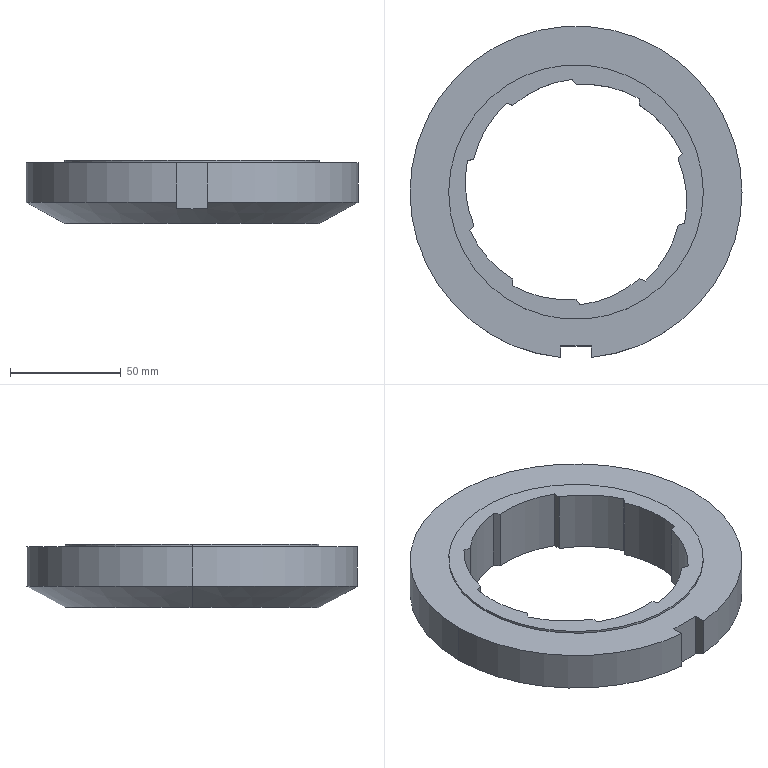Part | SolidWorks | features BaseBody 1, ICE 1 | 1 solid | 36 faces | box 150 x 149.673 x 28.6 mm | volume 237488 mm3 | cylinder 18 | plane 16 | cone 2 | commonest cylinder face diameters 100 x11 115 x4 150 x3
STEP:
#1=CARTESIAN_POINT('',(463.731,234.744,-713.193));
#2=VERTEX_POINT('',#1);
#3=CARTESIAN_POINT('',(578.731,234.744,-713.193));
#4=VERTEX_POINT('',#3);
#5=CARTESIAN_POINT('',(521.231,234.744,-713.193));
#6=DIRECTION('',(0.,0.,-1.));
#7=DIRECTION('',(-1.,0.,0.));
#8=AXIS2_PLACEMENT_3D('',#5,#6,#7);
#9=CIRCLE('',#8,57.5);
#10=EDGE_CURVE('',#2,#4,#9,.T.);
#11=ORIENTED_EDGE('',*,*,#10,.F.);
#12=CARTESIAN_POINT('',(446.231,234.744,-703.693));
#13=VERTEX_POINT('',#12);
#14=CARTESIAN_POINT('',(463.731,234.744,-713.193));
#15=DIRECTION('',(-0.8789,0.,0.4771));
#16=VECTOR('',#15,1000.);
#17=LINE('',#14,#16);
#18=EDGE_CURVE('',#2,#13,#17,.T.);
#19=ORIENTED_EDGE('',*,*,#18,.T.);
#20=CARTESIAN_POINT('',(596.231,234.744,-703.693));
#21=VERTEX_POINT('',#20);
#22=CARTESIAN_POINT('',(521.231,234.744,-703.693));
#23=DIRECTION('',(0.,0.,-1.));
#24=DIRECTION('',(-1.,0.,0.));
#25=AXIS2_PLACEMENT_3D('',#22,#23,#24);
#26=CIRCLE('',#25,75.);
#27=EDGE_CURVE('',#13,#21,#26,.T.);
#28=ORIENTED_EDGE('',*,*,#27,.T.);
#29=CARTESIAN_POINT('',(578.731,234.744,-713.193));
#30=DIRECTION('',(0.8789,0.,0.4771));
#31=VECTOR('',#30,1000.);
#32=LINE('',#29,#31);
#33=EDGE_CURVE('',#4,#21,#32,.T.);
#34=ORIENTED_EDGE('',*,*,#33,.F.);
#35=EDGE_LOOP('',(#11,#19,#28,#34));
#36=FACE_OUTER_BOUND('',#35,.T.);
#37=CARTESIAN_POINT('',(521.231,234.744,-713.193));
#38=DIRECTION('',(0.,0.,1.));
#39=DIRECTION('',(1.,0.,0.));
#40=AXIS2_PLACEMENT_3D('',#37,#38,#39);
#41=CONICAL_SURFACE('',#40,57.5,1.073);
#42=ADVANCED_FACE('',(#36),#41,.T.);
#43=CARTESIAN_POINT('',(578.731,234.744,-685.693));
#44=VERTEX_POINT('',#43);
#45=CARTESIAN_POINT('',(463.731,234.744,-685.693));
#46=VERTEX_POINT('',#45);
#47=CARTESIAN_POINT('',(521.231,234.744,-685.693));
#48=DIRECTION('',(0.,0.,1.));
#49=DIRECTION('',(1.,0.,0.));
#50=AXIS2_PLACEMENT_3D('',#47,#48,#49);
#51=CIRCLE('',#50,57.5);
#52=EDGE_CURVE('',#44,#46,#51,.T.);
#53=ORIENTED_EDGE('',*,*,#52,.T.);
#54=CARTESIAN_POINT('',(463.731,234.744,-684.693));
#55=VERTEX_POINT('',#54);
#56=CARTESIAN_POINT('',(463.731,234.744,-685.693));
#57=DIRECTION('',(0.,0.,1.));
#58=VECTOR('',#57,1000.);
#59=LINE('',#56,#58);
#60=EDGE_CURVE('',#46,#55,#59,.T.);
#61=ORIENTED_EDGE('',*,*,#60,.T.);
#62=CARTESIAN_POINT('',(578.731,234.744,-684.693));
#63=VERTEX_POINT('',#62);
#64=CARTESIAN_POINT('',(521.231,234.744,-684.693));
#65=DIRECTION('',(0.,0.,1.));
#66=DIRECTION('',(1.,0.,0.));
#67=AXIS2_PLACEMENT_3D('',#64,#65,#66);
#68=CIRCLE('',#67,57.5);
#69=EDGE_CURVE('',#63,#55,#68,.T.);
#70=ORIENTED_EDGE('',*,*,#69,.F.);
#71=CARTESIAN_POINT('',(578.731,234.744,-685.693));
#72=DIRECTION('',(0.,0.,1.));
#73=VECTOR('',#72,1000.);
#74=LINE('',#71,#73);
#75=EDGE_CURVE('',#44,#63,#74,.T.);
#76=ORIENTED_EDGE('',*,*,#75,.F.);
#77=EDGE_LOOP('',(#53,#61,#70,#76));
#78=FACE_OUTER_BOUND('',#77,.T.);
#79=CARTESIAN_POINT('',(521.231,234.744,-685.693));
#80=DIRECTION('',(0.,0.,1.));
#81=DIRECTION('',(1.,0.,0.));
#82=AXIS2_PLACEMENT_3D('',#79,#80,#81);
#83=CYLINDRICAL_SURFACE('',#82,57.5);
#84=ADVANCED_FACE('',(#78),#83,.T.);
#85=ORIENTED_EDGE('',*,*,#27,.F.);
#86=CARTESIAN_POINT('',(446.231,234.744,-685.693));
#87=VERTEX_POINT('',#86);
#88=CARTESIAN_POINT('',(446.231,234.744,-714.693));
#89=DIRECTION('',(0.,0.,1.));
#90=VECTOR('',#89,1000.);
#91=LINE('',#88,#90);
#92=EDGE_CURVE('',#13,#87,#91,.T.);
#93=ORIENTED_EDGE('',*,*,#92,.T.);
#94=CARTESIAN_POINT('',(596.231,234.744,-685.693));
#95=VERTEX_POINT('',#94);
#96=CARTESIAN_POINT('',(521.231,234.744,-685.693));
#97=DIRECTION('',(0.,0.,1.));
#98=DIRECTION('',(1.,0.,0.));
#99=AXIS2_PLACEMENT_3D('',#96,#97,#98);
#100=CIRCLE('',#99,75.);
#101=EDGE_CURVE('',#95,#87,#100,.T.);
#102=ORIENTED_EDGE('',*,*,#101,.F.);
#103=CARTESIAN_POINT('',(596.231,234.744,-714.693));
#104=DIRECTION('',(0.,0.,1.));
#105=VECTOR('',#104,1000.);
#106=LINE('',#103,#105);
#107=EDGE_CURVE('',#21,#95,#106,.T.);
#108=ORIENTED_EDGE('',*,*,#107,.F.);
#109=EDGE_LOOP('',(#85,#93,#102,#108));
#110=FACE_OUTER_BOUND('',#109,.T.);
#111=CARTESIAN_POINT('',(521.231,234.744,-714.693));
#112=DIRECTION('',(0.,0.,1.));
#113=DIRECTION('',(1.,0.,0.));
#114=AXIS2_PLACEMENT_3D('',#111,#112,#113);
#115=CYLINDRICAL_SURFACE('',#114,75.);
#116=ADVANCED_FACE('',(#110),#115,.T.);
#117=CARTESIAN_POINT('',(528.231,160.071,-703.693));
#118=VERTEX_POINT('',#117);
#119=CARTESIAN_POINT('',(521.231,234.744,-703.693));
#120=DIRECTION('',(0.,0.,-1.));
#121=DIRECTION('',(-1.,0.,0.));
#122=AXIS2_PLACEMENT_3D('',#119,#120,#121);
#123=CIRCLE('',#122,75.);
#124=EDGE_CURVE('',#21,#118,#123,.T.);
#125=ORIENTED_EDGE('',*,*,#124,.F.);
#126=ORIENTED_EDGE('',*,*,#107,.T.);
#127=CARTESIAN_POINT('',(528.231,160.071,-685.693));
#128=VERTEX_POINT('',#127);
#129=CARTESIAN_POINT('',(521.231,234.744,-685.693));
#130=DIRECTION('',(0.,0.,1.));
#131=DIRECTION('',(1.,0.,0.));
#132=AXIS2_PLACEMENT_3D('',#129,#130,#131);
#133=CIRCLE('',#132,75.);
#134=EDGE_CURVE('',#128,#95,#133,.T.);
#135=ORIENTED_EDGE('',*,*,#134,.F.);
#136=CARTESIAN_POINT('',(528.231,160.071,-714.693));
#137=DIRECTION('',(0.,0.,-1.));
#138=VECTOR('',#137,1000.);
#139=LINE('',#136,#138);
#140=EDGE_CURVE('',#128,#118,#139,.T.);
#141=ORIENTED_EDGE('',*,*,#140,.T.);
#142=EDGE_LOOP('',(#125,#126,#135,#141));
#143=FACE_OUTER_BOUND('',#142,.T.);
#144=CARTESIAN_POINT('',(521.231,234.744,-714.693));
#145=DIRECTION('',(0.,0.,1.));
#146=DIRECTION('',(1.,0.,0.));
#147=AXIS2_PLACEMENT_3D('',#144,#145,#146);
#148=CYLINDRICAL_SURFACE('',#147,75.);
#149=ADVANCED_FACE('',(#143),#148,.T.);
#150=CARTESIAN_POINT('',(471.242,239.027,-684.693));
#151=VERTEX_POINT('',#150);
#152=CARTESIAN_POINT('',(472.206,248.801,-684.693));
#153=VERTEX_POINT('',#152);
#154=CARTESIAN_POINT('',(521.242,239.027,-684.693));
#155=DIRECTION('',(0.,0.,-1.));
#156=DIRECTION('',(-1.,0.,0.));
#157=AXIS2_PLACEMENT_3D('',#154,#155,#156);
#158=CIRCLE('',#157,50.);
#159=EDGE_CURVE('',#151,#153,#158,.T.);
#160=ORIENTED_EDGE('',*,*,#159,.F.);
#161=CARTESIAN_POINT('',(471.242,239.027,-713.293));
#162=VERTEX_POINT('',#161);
#163=CARTESIAN_POINT('',(471.242,239.027,-608.693));
#164=DIRECTION('',(0.,0.,-1.));
#165=VECTOR('',#164,1000.);
#166=LINE('',#163,#165);
#167=EDGE_CURVE('',#151,#162,#166,.T.);
#168=ORIENTED_EDGE('',*,*,#167,.T.);
#169=CARTESIAN_POINT('',(472.206,248.801,-713.293));
#170=VERTEX_POINT('',#169);
#171=CARTESIAN_POINT('',(521.242,239.027,-713.293));
#172=DIRECTION('',(0.,0.,1.));
#173=DIRECTION('',(-1.,0.,0.));
#174=AXIS2_PLACEMENT_3D('',#171,#172,#173);
#175=CIRCLE('',#174,50.);
#176=EDGE_CURVE('',#170,#162,#175,.T.);
#177=ORIENTED_EDGE('',*,*,#176,.F.);
#178=CARTESIAN_POINT('',(472.206,248.801,-608.693));
#179=DIRECTION('',(0.,0.,-1.));
#180=VECTOR('',#179,1000.);
#181=LINE('',#178,#180);
#182=EDGE_CURVE('',#153,#170,#181,.T.);
#183=ORIENTED_EDGE('',*,*,#182,.F.);
#184=EDGE_LOOP('',(#160,#168,#177,#183));
#185=FACE_OUTER_BOUND('',#184,.T.);
#186=CARTESIAN_POINT('',(521.242,239.027,-608.693));
#187=DIRECTION('',(0.,0.,-1.));
#188=DIRECTION('',(-1.,0.,0.));
#189=AXIS2_PLACEMENT_3D('',#186,#187,#188);
#190=CYLINDRICAL_SURFACE('',#189,50.);
#191=ADVANCED_FACE('',(#185),#190,.F.);
#192=ORIENTED_EDGE('',*,*,#10,.T.);
#193=CARTESIAN_POINT('',(578.731,234.744,-713.293));
#194=VERTEX_POINT('',#193);
#195=CARTESIAN_POINT('',(578.731,234.744,-713.193));
#196=DIRECTION('',(0.,0.,-1.));
#197=VECTOR('',#196,1000.);
#198=LINE('',#195,#197);
#199=EDGE_CURVE('',#4,#194,#198,.T.);
#200=ORIENTED_EDGE('',*,*,#199,.T.);
#201=CARTESIAN_POINT('',(463.731,234.744,-713.293));
#202=VERTEX_POINT('',#201);
#203=CARTESIAN_POINT('',(521.231,234.744,-713.293));
#204=DIRECTION('',(0.,0.,-1.));
#205=DIRECTION('',(-1.,0.,0.));
#206=AXIS2_PLACEMENT_3D('',#203,#204,#205);
#207=CIRCLE('',#206,57.5);
#208=EDGE_CURVE('',#202,#194,#207,.T.);
#209=ORIENTED_EDGE('',*,*,#208,.F.);
#210=CARTESIAN_POINT('',(463.731,234.744,-713.193));
#211=DIRECTION('',(0.,0.,-1.));
#212=VECTOR('',#211,1000.);
#213=LINE('',#210,#212);
#214=EDGE_CURVE('',#2,#202,#213,.T.);
#215=ORIENTED_EDGE('',*,*,#214,.F.);
#216=EDGE_LOOP('',(#192,#200,#209,#215));
#217=FACE_OUTER_BOUND('',#216,.T.);
#218=CARTESIAN_POINT('',(521.231,234.744,-713.193));
#219=DIRECTION('',(0.,0.,-1.));
#220=DIRECTION('',(-1.,0.,0.));
#221=AXIS2_PLACEMENT_3D('',#218,#219,#220);
#222=CYLINDRICAL_SURFACE('',#221,57.5);
#223=ADVANCED_FACE('',(#217),#222,.T.);
#224=ORIENTED_EDGE('',*,*,#199,.F.);
#225=CARTESIAN_POINT('',(521.231,234.744,-713.193));
#226=DIRECTION('',(0.,0.,-1.));
#227=DIRECTION('',(-1.,0.,0.));
#228=AXIS2_PLACEMENT_3D('',#225,#226,#227);
#229=CIRCLE('',#228,57.5);
#230=EDGE_CURVE('',#4,#2,#229,.T.);
#231=ORIENTED_EDGE('',*,*,#230,.T.);
#232=ORIENTED_EDGE('',*,*,#214,.T.);
#233=CARTESIAN_POINT('',(521.231,234.744,-713.293));
#234=DIRECTION('',(0.,0.,-1.));
#235=DIRECTION('',(-1.,0.,0.));
#236=AXIS2_PLACEMENT_3D('',#233,#234,#235);
#237=CIRCLE('',#236,57.5);
#238=EDGE_CURVE('',#194,#202,#237,.T.);
#239=ORIENTED_EDGE('',*,*,#238,.F.);
#240=EDGE_LOOP('',(#224,#231,#232,#239));
#241=FACE_OUTER_BOUND('',#240,.T.);
#242=CARTESIAN_POINT('',(521.231,234.744,-713.193));
#243=DIRECTION('',(0.,0.,-1.));
#244=DIRECTION('',(-1.,0.,0.));
#245=AXIS2_PLACEMENT_3D('',#242,#243,#244);
#246=CYLINDRICAL_SURFACE('',#245,57.5);
#247=ADVANCED_FACE('',(#241),#246,.T.);
#248=CARTESIAN_POINT('',(521.231,186.244,-713.293));
#249=VERTEX_POINT('',#248);
#250=CARTESIAN_POINT('',(523.011,183.775,-713.293));
#251=VERTEX_POINT('',#250);
#252=CARTESIAN_POINT('',(523.011,183.775,-713.293));
#253=DIRECTION('',(0.5848,-0.8112,0.));
#254=VECTOR('',#253,1000.);
#255=LINE('',#252,#254);
#256=EDGE_CURVE('',#249,#251,#255,.T.);
#257=ORIENTED_EDGE('',*,*,#256,.F.);
#258=CARTESIAN_POINT('',(521.231,186.244,-684.693));
#259=VERTEX_POINT('',#258);
#260=CARTESIAN_POINT('',(521.231,186.244,-608.693));
#261=DIRECTION('',(0.,0.,-1.));
#262=VECTOR('',#261,1000.);
#263=LINE('',#260,#262);
#264=EDGE_CURVE('',#259,#249,#263,.T.);
#265=ORIENTED_EDGE('',*,*,#264,.F.);
#266=CARTESIAN_POINT('',(523.011,183.775,-684.693));
#267=VERTEX_POINT('',#266);
#268=CARTESIAN_POINT('',(498.224,218.158,-684.693));
#269=DIRECTION('',(-0.5848,0.8112,0.));
#270=VECTOR('',#269,1000.);
#271=LINE('',#268,#270);
#272=EDGE_CURVE('',#267,#259,#271,.T.);
#273=ORIENTED_EDGE('',*,*,#272,.F.);
#274=CARTESIAN_POINT('',(523.011,183.775,-608.693));
#275=DIRECTION('',(0.,0.,-1.));
#276=VECTOR('',#275,1000.);
#277=LINE('',#274,#276);
#278=EDGE_CURVE('',#267,#251,#277,.T.);
#279=ORIENTED_EDGE('',*,*,#278,.T.);
#280=EDGE_LOOP('',(#257,#265,#273,#279));
#281=FACE_OUTER_BOUND('',#280,.T.);
#282=CARTESIAN_POINT('',(523.011,183.775,-608.693));
#283=DIRECTION('',(-0.8112,-0.5848,0.));
#284=DIRECTION('',(-0.5848,0.8112,0.));
#285=AXIS2_PLACEMENT_3D('',#282,#283,#284);
#286=PLANE('',#285);
#287=ADVANCED_FACE('',(#281),#286,.F.);
#288=CARTESIAN_POINT('',(492.712,192.463,-713.293));
#289=VERTEX_POINT('',#288);
#290=CARTESIAN_POINT('',(517.16,236.078,-713.293));
#291=DIRECTION('',(0.,0.,1.));
#292=DIRECTION('',(-1.,0.,0.));
#293=AXIS2_PLACEMENT_3D('',#290,#291,#292);
#294=CIRCLE('',#293,50.);
#295=EDGE_CURVE('',#289,#249,#294,.T.);
#296=ORIENTED_EDGE('',*,*,#295,.F.);
#297=CARTESIAN_POINT('',(492.712,192.463,-684.693));
#298=VERTEX_POINT('',#297);
#299=CARTESIAN_POINT('',(492.712,192.463,-608.693));
#300=DIRECTION('',(0.,0.,-1.));
#301=VECTOR('',#300,1000.);
#302=LINE('',#299,#301);
#303=EDGE_CURVE('',#298,#289,#302,.T.);
#304=ORIENTED_EDGE('',*,*,#303,.F.);
#305=CARTESIAN_POINT('',(517.16,236.078,-684.693));
#306=DIRECTION('',(0.,0.,-1.));
#307=DIRECTION('',(-1.,0.,0.));
#308=AXIS2_PLACEMENT_3D('',#305,#306,#307);
#309=CIRCLE('',#308,50.);
#310=EDGE_CURVE('',#259,#298,#309,.T.);
#311=ORIENTED_EDGE('',*,*,#310,.F.);
#312=ORIENTED_EDGE('',*,*,#264,.T.);
#313=EDGE_LOOP('',(#296,#304,#311,#312));
#314=FACE_OUTER_BOUND('',#313,.T.);
#315=CARTESIAN_POINT('',(517.16,236.078,-608.693));
#316=DIRECTION('',(0.,0.,-1.));
#317=DIRECTION('',(-1.,0.,0.));
#318=AXIS2_PLACEMENT_3D('',#315,#316,#317);
#319=CYLINDRICAL_SURFACE('',#318,50.);
#320=ADVANCED_FACE('',(#314),#319,.F.);
#321=CARTESIAN_POINT('',(475.104,219.757,-713.293));
#322=VERTEX_POINT('',#321);
#323=CARTESIAN_POINT('',(473.306,217.301,-713.293));
#324=VERTEX_POINT('',#323);
#325=CARTESIAN_POINT('',(473.306,217.301,-713.293));
#326=DIRECTION('',(-0.5908,-0.8068,0.));
#327=VECTOR('',#326,1000.);
#328=LINE('',#325,#327);
#329=EDGE_CURVE('',#322,#324,#328,.T.);
#330=ORIENTED_EDGE('',*,*,#329,.F.);
#331=CARTESIAN_POINT('',(475.104,219.757,-684.693));
#332=VERTEX_POINT('',#331);
#333=CARTESIAN_POINT('',(475.104,219.757,-608.693));
#334=DIRECTION('',(0.,0.,-1.));
#335=VECTOR('',#334,1000.);
#336=LINE('',#333,#335);
#337=EDGE_CURVE('',#332,#322,#336,.T.);
#338=ORIENTED_EDGE('',*,*,#337,.F.);
#339=CARTESIAN_POINT('',(473.306,217.301,-684.693));
#340=VERTEX_POINT('',#339);
#341=CARTESIAN_POINT('',(498.347,251.5,-684.693));
#342=DIRECTION('',(0.5908,0.8068,0.));
#343=VECTOR('',#342,1000.);
#344=LINE('',#341,#343);
#345=EDGE_CURVE('',#340,#332,#344,.T.);
#346=ORIENTED_EDGE('',*,*,#345,.F.);
#347=CARTESIAN_POINT('',(473.306,217.301,-608.693));
#348=DIRECTION('',(0.,0.,-1.));
#349=VECTOR('',#348,1000.);
#350=LINE('',#347,#349);
#351=EDGE_CURVE('',#340,#324,#350,.T.);
#352=ORIENTED_EDGE('',*,*,#351,.T.);
#353=EDGE_LOOP('',(#330,#338,#346,#352));
#354=FACE_OUTER_BOUND('',#353,.T.);
#355=CARTESIAN_POINT('',(473.306,217.301,-608.693));
#356=DIRECTION('',(-0.8068,0.5908,0.));
#357=DIRECTION('',(0.5908,0.8068,0.));
#358=AXIS2_PLACEMENT_3D('',#355,#356,#357);
#359=PLANE('',#358);
#360=ADVANCED_FACE('',(#354),#359,.F.);
#361=CARTESIAN_POINT('',(492.723,273.981,-713.293));
#362=VERTEX_POINT('',#361);
#363=CARTESIAN_POINT('',(489.832,274.933,-713.293));
#364=VERTEX_POINT('',#363);
#365=CARTESIAN_POINT('',(489.832,274.933,-713.293));
#366=DIRECTION('',(-0.9499,0.3125,0.));
#367=VECTOR('',#366,1000.);
#368=LINE('',#365,#367);
#369=EDGE_CURVE('',#362,#364,#368,.T.);
#370=ORIENTED_EDGE('',*,*,#369,.F.);
#371=CARTESIAN_POINT('',(492.723,273.981,-684.693));
#372=VERTEX_POINT('',#371);
#373=CARTESIAN_POINT('',(492.723,273.981,-608.693));
#374=DIRECTION('',(0.,0.,-1.));
#375=VECTOR('',#374,1000.);
#376=LINE('',#373,#375);
#377=EDGE_CURVE('',#372,#362,#376,.T.);
#378=ORIENTED_EDGE('',*,*,#377,.F.);
#379=CARTESIAN_POINT('',(489.832,274.933,-684.693));
#380=VERTEX_POINT('',#379);
#381=CARTESIAN_POINT('',(530.095,261.686,-684.693));
#382=DIRECTION('',(0.9499,-0.3125,0.));
#383=VECTOR('',#382,1000.);
#384=LINE('',#381,#383);
#385=EDGE_CURVE('',#380,#372,#384,.T.);
#386=ORIENTED_EDGE('',*,*,#385,.F.);
#387=CARTESIAN_POINT('',(489.832,274.933,-608.693));
#388=DIRECTION('',(0.,0.,-1.));
#389=VECTOR('',#388,1000.);
#390=LINE('',#387,#389);
#391=EDGE_CURVE('',#380,#364,#390,.T.);
#392=ORIENTED_EDGE('',*,*,#391,.T.);
#393=EDGE_LOOP('',(#370,#378,#386,#392));
#394=FACE_OUTER_BOUND('',#393,.T.);
#395=CARTESIAN_POINT('',(489.832,274.933,-608.693));
#396=DIRECTION('',(0.3125,0.9499,0.));
#397=DIRECTION('',(0.9499,-0.3125,0.));
#398=AXIS2_PLACEMENT_3D('',#395,#396,#397);
#399=PLANE('',#398);
#400=ADVANCED_FACE('',(#394),#399,.F.);
#401=CARTESIAN_POINT('',(549.738,273.981,-713.293));
#402=VERTEX_POINT('',#401);
#403=CARTESIAN_POINT('',(549.749,277.025,-713.293));
#404=VERTEX_POINT('',#403);
#405=CARTESIAN_POINT('',(549.749,277.025,-713.293));
#406=DIRECTION('',(0.003697,1.,0.));
#407=VECTOR('',#406,1000.);
#408=LINE('',#405,#407);
#409=EDGE_CURVE('',#402,#404,#408,.T.);
#410=ORIENTED_EDGE('',*,*,#409,.F.);
#411=CARTESIAN_POINT('',(549.738,273.981,-684.693));
#412=VERTEX_POINT('',#411);
#413=CARTESIAN_POINT('',(549.738,273.981,-608.693));
#414=DIRECTION('',(0.,0.,-1.));
#415=VECTOR('',#414,1000.);
#416=LINE('',#413,#415);
#417=EDGE_CURVE('',#412,#402,#416,.T.);
#418=ORIENTED_EDGE('',*,*,#417,.F.);
#419=CARTESIAN_POINT('',(549.749,277.025,-684.693));
#420=VERTEX_POINT('',#419);
#421=CARTESIAN_POINT('',(549.593,234.639,-684.693));
#422=DIRECTION('',(-0.003697,-1.,0.));
#423=VECTOR('',#422,1000.);
#424=LINE('',#421,#423);
#425=EDGE_CURVE('',#420,#412,#424,.T.);
#426=ORIENTED_EDGE('',*,*,#425,.F.);
#427=CARTESIAN_POINT('',(549.749,277.025,-608.693));
#428=DIRECTION('',(0.,0.,-1.));
#429=VECTOR('',#428,1000.);
#430=LINE('',#427,#429);
#431=EDGE_CURVE('',#420,#404,#430,.T.);
#432=ORIENTED_EDGE('',*,*,#431,.T.);
#433=EDGE_LOOP('',(#410,#418,#426,#432));
#434=FACE_OUTER_BOUND('',#433,.T.);
#435=CARTESIAN_POINT('',(549.749,277.025,-608.693));
#436=DIRECTION('',(1.,-0.003697,0.));
#437=DIRECTION('',(-0.003697,-1.,0.));
#438=AXIS2_PLACEMENT_3D('',#435,#436,#437);
#439=PLANE('',#438);
#440=ADVANCED_FACE('',(#434),#439,.F.);
#441=CARTESIAN_POINT('',(567.357,219.757,-713.293));
#442=VERTEX_POINT('',#441);
#443=CARTESIAN_POINT('',(570.255,220.686,-713.293));
#444=VERTEX_POINT('',#443);
#445=CARTESIAN_POINT('',(570.255,220.686,-713.293));
#446=DIRECTION('',(0.9522,0.3055,0.));
#447=VECTOR('',#446,1000.);
#448=LINE('',#445,#447);
#449=EDGE_CURVE('',#442,#444,#448,.T.);
#450=ORIENTED_EDGE('',*,*,#449,.F.);
#451=CARTESIAN_POINT('',(567.357,219.757,-684.693));
#452=VERTEX_POINT('',#451);
#453=CARTESIAN_POINT('',(567.357,219.757,-608.693));
#454=DIRECTION('',(0.,0.,-1.));
#455=VECTOR('',#454,1000.);
#456=LINE('',#453,#455);
#457=EDGE_CURVE('',#452,#442,#456,.T.);
#458=ORIENTED_EDGE('',*,*,#457,.F.);
#459=CARTESIAN_POINT('',(570.255,220.686,-684.693));
#460=VERTEX_POINT('',#459);
#461=CARTESIAN_POINT('',(529.895,207.738,-684.693));
#462=DIRECTION('',(-0.9522,-0.3055,0.));
#463=VECTOR('',#462,1000.);
#464=LINE('',#461,#463);
#465=EDGE_CURVE('',#460,#452,#464,.T.);
#466=ORIENTED_EDGE('',*,*,#465,.F.);
#467=CARTESIAN_POINT('',(570.255,220.686,-608.693));
#468=DIRECTION('',(0.,0.,-1.));
#469=VECTOR('',#468,1000.);
#470=LINE('',#467,#469);
#471=EDGE_CURVE('',#460,#444,#470,.T.);
#472=ORIENTED_EDGE('',*,*,#471,.T.);
#473=EDGE_LOOP('',(#450,#458,#466,#472));
#474=FACE_OUTER_BOUND('',#473,.T.);
#475=CARTESIAN_POINT('',(570.255,220.686,-608.693));
#476=DIRECTION('',(0.3055,-0.9522,0.));
#477=DIRECTION('',(-0.9522,-0.3055,0.));
#478=AXIS2_PLACEMENT_3D('',#475,#476,#477);
#479=PLANE('',#478);
#480=ADVANCED_FACE('',(#474),#479,.F.);
#481=CARTESIAN_POINT('',(492.723,195.507,-713.293));
#482=VERTEX_POINT('',#481);
#483=CARTESIAN_POINT('',(518.722,238.216,-713.293));
#484=DIRECTION('',(0.,0.,1.));
#485=DIRECTION('',(-1.,0.,0.));
#486=AXIS2_PLACEMENT_3D('',#483,#484,#485);
#487=CIRCLE('',#486,50.);
#488=EDGE_CURVE('',#324,#482,#487,.T.);
#489=ORIENTED_EDGE('',*,*,#488,.F.);
#490=ORIENTED_EDGE('',*,*,#351,.F.);
#491=CARTESIAN_POINT('',(492.723,195.507,-684.693));
#492=VERTEX_POINT('',#491);
#493=CARTESIAN_POINT('',(518.722,238.216,-684.693));
#494=DIRECTION('',(0.,0.,-1.));
#495=DIRECTION('',(-1.,0.,0.));
#496=AXIS2_PLACEMENT_3D('',#493,#494,#495);
#497=CIRCLE('',#496,50.);
#498=EDGE_CURVE('',#492,#340,#497,.T.);
#499=ORIENTED_EDGE('',*,*,#498,.F.);
#500=CARTESIAN_POINT('',(492.723,195.507,-608.693));
#501=DIRECTION('',(0.,0.,-1.));
#502=VECTOR('',#501,1000.);
#503=LINE('',#500,#502);
#504=EDGE_CURVE('',#492,#482,#503,.T.);
#505=ORIENTED_EDGE('',*,*,#504,.T.);
#506=EDGE_LOOP('',(#489,#490,#499,#505));
#507=FACE_OUTER_BOUND('',#506,.T.);
#508=CARTESIAN_POINT('',(518.722,238.216,-608.693));
#509=DIRECTION('',(0.,0.,-1.));
#510=DIRECTION('',(-1.,0.,0.));
#511=AXIS2_PLACEMENT_3D('',#508,#509,#510);
#512=CYLINDRICAL_SURFACE('',#511,50.);
#513=ADVANCED_FACE('',(#507),#512,.F.);
#514=CARTESIAN_POINT('',(475.104,249.731,-713.293));
#515=VERTEX_POINT('',#514);
#516=CARTESIAN_POINT('',(523.757,238.203,-713.293));
#517=DIRECTION('',(0.,0.,1.));
#518=DIRECTION('',(-1.,0.,0.));
#519=AXIS2_PLACEMENT_3D('',#516,#517,#518);
#520=CIRCLE('',#519,50.);
#521=EDGE_CURVE('',#364,#515,#520,.T.);
#522=ORIENTED_EDGE('',*,*,#521,.F.);
#523=ORIENTED_EDGE('',*,*,#391,.F.);
#524=CARTESIAN_POINT('',(475.104,249.731,-684.693));
#525=VERTEX_POINT('',#524);
#526=CARTESIAN_POINT('',(523.757,238.203,-684.693));
#527=DIRECTION('',(0.,0.,-1.));
#528=DIRECTION('',(-1.,0.,0.));
#529=AXIS2_PLACEMENT_3D('',#526,#527,#528);
#530=CIRCLE('',#529,50.);
#531=EDGE_CURVE('',#525,#380,#530,.T.);
#532=ORIENTED_EDGE('',*,*,#531,.F.);
#533=CARTESIAN_POINT('',(475.104,249.731,-608.693));
#534=DIRECTION('',(0.,0.,-1.));
#535=VECTOR('',#534,1000.);
#536=LINE('',#533,#535);
#537=EDGE_CURVE('',#525,#515,#536,.T.);
#538=ORIENTED_EDGE('',*,*,#537,.T.);
#539=EDGE_LOOP('',(#522,#523,#532,#538));
#540=FACE_OUTER_BOUND('',#539,.T.);
#541=CARTESIAN_POINT('',(523.757,238.203,-608.693));
#542=DIRECTION('',(0.,0.,-1.));
#543=DIRECTION('',(-1.,0.,0.));
#544=AXIS2_PLACEMENT_3D('',#541,#542,#543);
#545=CYLINDRICAL_SURFACE('',#544,50.);
#546=ADVANCED_FACE('',(#540),#545,.F.);
#547=CARTESIAN_POINT('',(521.231,283.244,-713.293));
#548=VERTEX_POINT('',#547);
#549=CARTESIAN_POINT('',(525.301,233.41,-713.293));
#550=DIRECTION('',(0.,0.,1.));
#551=DIRECTION('',(-1.,0.,0.));
#552=AXIS2_PLACEMENT_3D('',#549,#550,#551);
#553=CIRCLE('',#552,50.);
#554=EDGE_CURVE('',#404,#548,#553,.T.);
#555=ORIENTED_EDGE('',*,*,#554,.F.);
#556=ORIENTED_EDGE('',*,*,#431,.F.);
#557=CARTESIAN_POINT('',(521.231,283.244,-684.693));
#558=VERTEX_POINT('',#557);
#559=CARTESIAN_POINT('',(525.301,233.41,-684.693));
#560=DIRECTION('',(0.,0.,-1.));
#561=DIRECTION('',(-1.,0.,0.));
#562=AXIS2_PLACEMENT_3D('',#559,#560,#561);
#563=CIRCLE('',#562,50.);
#564=EDGE_CURVE('',#558,#420,#563,.T.);
#565=ORIENTED_EDGE('',*,*,#564,.F.);
#566=CARTESIAN_POINT('',(521.231,283.244,-608.693));
#567=DIRECTION('',(0.,0.,-1.));
#568=VECTOR('',#567,1000.);
#569=LINE('',#566,#568);
#570=EDGE_CURVE('',#558,#548,#569,.T.);
#571=ORIENTED_EDGE('',*,*,#570,.T.);
#572=EDGE_LOOP('',(#555,#556,#565,#571));
#573=FACE_OUTER_BOUND('',#572,.T.);
#574=CARTESIAN_POINT('',(525.301,233.41,-608.693));
#575=DIRECTION('',(0.,0.,-1.));
#576=DIRECTION('',(-1.,0.,0.));
#577=AXIS2_PLACEMENT_3D('',#574,#575,#576);
#578=CYLINDRICAL_SURFACE('',#577,50.);
#579=ADVANCED_FACE('',(#573),#578,.F.);
#580=CARTESIAN_POINT('',(567.357,249.731,-713.293));
#581=VERTEX_POINT('',#580);
#582=CARTESIAN_POINT('',(521.22,230.461,-713.293));
#583=DIRECTION('',(0.,0.,1.));
#584=DIRECTION('',(-1.,0.,0.));
#585=AXIS2_PLACEMENT_3D('',#582,#583,#584);
#586=CIRCLE('',#585,50.);
#587=EDGE_CURVE('',#444,#581,#586,.T.);
#588=ORIENTED_EDGE('',*,*,#587,.F.);
#589=ORIENTED_EDGE('',*,*,#471,.F.);
#590=CARTESIAN_POINT('',(567.357,249.731,-684.693));
#591=VERTEX_POINT('',#590);
#592=CARTESIAN_POINT('',(521.22,230.461,-684.693));
#593=DIRECTION('',(0.,0.,-1.));
#594=DIRECTION('',(-1.,0.,0.));
#595=AXIS2_PLACEMENT_3D('',#592,#593,#594);
#596=CIRCLE('',#595,50.);
#597=EDGE_CURVE('',#591,#460,#596,.T.);
#598=ORIENTED_EDGE('',*,*,#597,.F.);
#599=CARTESIAN_POINT('',(567.357,249.731,-608.693));
#600=DIRECTION('',(0.,0.,-1.));
#601=VECTOR('',#600,1000.);
#602=LINE('',#599,#601);
#603=EDGE_CURVE('',#591,#581,#602,.T.);
#604=ORIENTED_EDGE('',*,*,#603,.T.);
#605=EDGE_LOOP('',(#588,#589,#598,#604));
#606=FACE_OUTER_BOUND('',#605,.T.);
#607=CARTESIAN_POINT('',(521.22,230.461,-608.693));
#608=DIRECTION('',(0.,0.,-1.));
#609=DIRECTION('',(-1.,0.,0.));
#610=AXIS2_PLACEMENT_3D('',#607,#608,#609);
#611=CYLINDRICAL_SURFACE('',#610,50.);
#612=ADVANCED_FACE('',(#606),#611,.F.);
#613=CARTESIAN_POINT('',(472.206,248.801,-713.293));
#614=DIRECTION('',(-0.9522,-0.3055,0.));
#615=VECTOR('',#614,1000.);
#616=LINE('',#613,#615);
#617=EDGE_CURVE('',#515,#170,#616,.T.);
#618=ORIENTED_EDGE('',*,*,#617,.F.);
#619=ORIENTED_EDGE('',*,*,#537,.F.);
#620=CARTESIAN_POINT('',(512.566,261.75,-684.693));
#621=DIRECTION('',(0.9522,0.3055,0.));
#622=VECTOR('',#621,1000.);
#623=LINE('',#620,#622);
#624=EDGE_CURVE('',#153,#525,#623,.T.);
#625=ORIENTED_EDGE('',*,*,#624,.F.);
#626=ORIENTED_EDGE('',*,*,#182,.T.);
#627=EDGE_LOOP('',(#618,#619,#625,#626));
#628=FACE_OUTER_BOUND('',#627,.T.);
#629=CARTESIAN_POINT('',(472.206,248.801,-608.693));
#630=DIRECTION('',(-0.3055,0.9522,0.));
#631=DIRECTION('',(0.9522,0.3055,0.));
#632=AXIS2_PLACEMENT_3D('',#629,#630,#631);
#633=PLANE('',#632);
#634=ADVANCED_FACE('',(#628),#633,.F.);
#635=CARTESIAN_POINT('',(519.451,285.713,-713.293));
#636=VERTEX_POINT('',#635);
#637=CARTESIAN_POINT('',(519.451,285.713,-713.293));
#638=DIRECTION('',(-0.5848,0.8112,0.));
#639=VECTOR('',#638,1000.);
#640=LINE('',#637,#639);
#641=EDGE_CURVE('',#548,#636,#640,.T.);
#642=ORIENTED_EDGE('',*,*,#641,.F.);
#643=ORIENTED_EDGE('',*,*,#570,.F.);
#644=CARTESIAN_POINT('',(519.451,285.713,-684.693));
#645=VERTEX_POINT('',#644);
#646=CARTESIAN_POINT('',(544.238,251.33,-684.693));
#647=DIRECTION('',(0.5848,-0.8112,0.));
#648=VECTOR('',#647,1000.);
#649=LINE('',#646,#648);
#650=EDGE_CURVE('',#645,#558,#649,.T.);
#651=ORIENTED_EDGE('',*,*,#650,.F.);
#652=CARTESIAN_POINT('',(519.451,285.713,-608.693));
#653=DIRECTION('',(0.,0.,-1.));
#654=VECTOR('',#653,1000.);
#655=LINE('',#652,#654);
#656=EDGE_CURVE('',#645,#636,#655,.T.);
#657=ORIENTED_EDGE('',*,*,#656,.T.);
#658=EDGE_LOOP('',(#642,#643,#651,#657));
#659=FACE_OUTER_BOUND('',#658,.T.);
#660=CARTESIAN_POINT('',(519.451,285.713,-608.693));
#661=DIRECTION('',(0.8112,0.5848,0.));
#662=DIRECTION('',(0.5848,-0.8112,0.));
#663=AXIS2_PLACEMENT_3D('',#660,#661,#662);
#664=PLANE('',#663);
#665=ADVANCED_FACE('',(#659),#664,.F.);
#666=CARTESIAN_POINT('',(569.155,252.187,-713.293));
#667=VERTEX_POINT('',#666);
#668=CARTESIAN_POINT('',(569.155,252.187,-713.293));
#669=DIRECTION('',(0.5908,0.8068,0.));
#670=VECTOR('',#669,1000.);
#671=LINE('',#668,#670);
#672=EDGE_CURVE('',#581,#667,#671,.T.);
#673=ORIENTED_EDGE('',*,*,#672,.F.);
#674=ORIENTED_EDGE('',*,*,#603,.F.);
#675=CARTESIAN_POINT('',(569.155,252.187,-684.693));
#676=VERTEX_POINT('',#675);
#677=CARTESIAN_POINT('',(544.114,217.988,-684.693));
#678=DIRECTION('',(-0.5908,-0.8068,0.));
#679=VECTOR('',#678,1000.);
#680=LINE('',#677,#679);
#681=EDGE_CURVE('',#676,#591,#680,.T.);
#682=ORIENTED_EDGE('',*,*,#681,.F.);
#683=CARTESIAN_POINT('',(569.155,252.187,-608.693));
#684=DIRECTION('',(0.,0.,-1.));
#685=VECTOR('',#684,1000.);
#686=LINE('',#683,#685);
#687=EDGE_CURVE('',#676,#667,#686,.T.);
#688=ORIENTED_EDGE('',*,*,#687,.T.);
#689=EDGE_LOOP('',(#673,#674,#682,#688));
#690=FACE_OUTER_BOUND('',#689,.T.);
#691=CARTESIAN_POINT('',(569.155,252.187,-608.693));
#692=DIRECTION('',(0.8068,-0.5908,0.));
#693=DIRECTION('',(-0.5908,-0.8068,0.));
#694=AXIS2_PLACEMENT_3D('',#691,#692,#693);
#695=PLANE('',#694);
#696=ADVANCED_FACE('',(#690),#695,.F.);
#697=CARTESIAN_POINT('',(549.738,195.507,-713.293));
#698=VERTEX_POINT('',#697);
#699=CARTESIAN_POINT('',(552.629,194.555,-713.293));
#700=VERTEX_POINT('',#699);
#701=CARTESIAN_POINT('',(552.629,194.555,-713.293));
#702=DIRECTION('',(0.9499,-0.3125,0.));
#703=VECTOR('',#702,1000.);
#704=LINE('',#701,#703);
#705=EDGE_CURVE('',#698,#700,#704,.T.);
#706=ORIENTED_EDGE('',*,*,#705,.F.);
#707=CARTESIAN_POINT('',(549.738,195.507,-684.693));
#708=VERTEX_POINT('',#707);
#709=CARTESIAN_POINT('',(549.738,195.507,-608.693));
#710=DIRECTION('',(0.,0.,-1.));
#711=VECTOR('',#710,1000.);
#712=LINE('',#709,#711);
#713=EDGE_CURVE('',#708,#698,#712,.T.);
#714=ORIENTED_EDGE('',*,*,#713,.F.);
#715=CARTESIAN_POINT('',(552.629,194.555,-684.693));
#716=VERTEX_POINT('',#715);
#717=CARTESIAN_POINT('',(512.367,207.802,-684.693));
#718=DIRECTION('',(-0.9499,0.3125,0.));
#719=VECTOR('',#718,1000.);
#720=LINE('',#717,#719);
#721=EDGE_CURVE('',#716,#708,#720,.T.);
#722=ORIENTED_EDGE('',*,*,#721,.F.);
#723=CARTESIAN_POINT('',(552.629,194.555,-608.693));
#724=DIRECTION('',(0.,0.,-1.));
#725=VECTOR('',#724,1000.);
#726=LINE('',#723,#725);
#727=EDGE_CURVE('',#716,#700,#726,.T.);
#728=ORIENTED_EDGE('',*,*,#727,.T.);
#729=EDGE_LOOP('',(#706,#714,#722,#728));
#730=FACE_OUTER_BOUND('',#729,.T.);
#731=CARTESIAN_POINT('',(552.629,194.555,-608.693));
#732=DIRECTION('',(-0.3125,-0.9499,0.));
#733=DIRECTION('',(-0.9499,0.3125,0.));
#734=AXIS2_PLACEMENT_3D('',#731,#732,#733);
#735=PLANE('',#734);
#736=ADVANCED_FACE('',(#730),#735,.F.);
#737=ORIENTED_EDGE('',*,*,#167,.F.);
#738=CARTESIAN_POINT('',(521.242,239.027,-684.693));
#739=DIRECTION('',(0.,0.,-1.));
#740=DIRECTION('',(-1.,0.,0.));
#741=AXIS2_PLACEMENT_3D('',#738,#739,#740);
#742=CIRCLE('',#741,50.);
#743=EDGE_CURVE('',#332,#151,#742,.T.);
#744=ORIENTED_EDGE('',*,*,#743,.F.);
#745=ORIENTED_EDGE('',*,*,#337,.T.);
#746=CARTESIAN_POINT('',(521.242,239.027,-713.293));
#747=DIRECTION('',(0.,0.,1.));
#748=DIRECTION('',(-1.,0.,0.));
#749=AXIS2_PLACEMENT_3D('',#746,#747,#748);
#750=CIRCLE('',#749,50.);
#751=EDGE_CURVE('',#162,#322,#750,.T.);
#752=ORIENTED_EDGE('',*,*,#751,.F.);
#753=EDGE_LOOP('',(#737,#744,#745,#752));
#754=FACE_OUTER_BOUND('',#753,.T.);
#755=CARTESIAN_POINT('',(521.242,239.027,-608.693));
#756=DIRECTION('',(0.,0.,-1.));
#757=DIRECTION('',(-1.,0.,0.));
#758=AXIS2_PLACEMENT_3D('',#755,#756,#757);
#759=CYLINDRICAL_SURFACE('',#758,50.);
#760=ADVANCED_FACE('',(#754),#759,.F.);
#761=CARTESIAN_POINT('',(525.308,236.057,-713.293));
#762=DIRECTION('',(0.,0.,1.));
#763=DIRECTION('',(-1.,0.,0.));
#764=AXIS2_PLACEMENT_3D('',#761,#762,#763);
#765=CIRCLE('',#764,50.);
#766=EDGE_CURVE('',#636,#362,#765,.T.);
#767=ORIENTED_EDGE('',*,*,#766,.F.);
#768=ORIENTED_EDGE('',*,*,#656,.F.);
#769=CARTESIAN_POINT('',(525.308,236.057,-684.693));
#770=DIRECTION('',(0.,0.,-1.));
#771=DIRECTION('',(-1.,0.,0.));
#772=AXIS2_PLACEMENT_3D('',#769,#770,#771);
#773=CIRCLE('',#772,50.);
#774=EDGE_CURVE('',#372,#645,#773,.T.);
#775=ORIENTED_EDGE('',*,*,#774,.F.);
#776=ORIENTED_EDGE('',*,*,#377,.T.);
#777=EDGE_LOOP('',(#767,#768,#775,#776));
#778=FACE_OUTER_BOUND('',#777,.T.);
#779=CARTESIAN_POINT('',(525.308,236.057,-608.693));
#780=DIRECTION('',(0.,0.,-1.));
#781=DIRECTION('',(-1.,0.,0.));
#782=AXIS2_PLACEMENT_3D('',#779,#780,#781);
#783=CYLINDRICAL_SURFACE('',#782,50.);
#784=ADVANCED_FACE('',(#778),#783,.F.);
#785=CARTESIAN_POINT('',(523.739,231.272,-713.293));
#786=DIRECTION('',(0.,0.,1.));
#787=DIRECTION('',(-1.,0.,0.));
#788=AXIS2_PLACEMENT_3D('',#785,#786,#787);
#789=CIRCLE('',#788,50.);
#790=EDGE_CURVE('',#667,#402,#789,.T.);
#791=ORIENTED_EDGE('',*,*,#790,.F.);
#792=ORIENTED_EDGE('',*,*,#687,.F.);
#793=CARTESIAN_POINT('',(523.739,231.272,-684.693));
#794=DIRECTION('',(0.,0.,-1.));
#795=DIRECTION('',(-1.,0.,0.));
#796=AXIS2_PLACEMENT_3D('',#793,#794,#795);
#797=CIRCLE('',#796,50.);
#798=EDGE_CURVE('',#412,#676,#797,.T.);
#799=ORIENTED_EDGE('',*,*,#798,.F.);
#800=ORIENTED_EDGE('',*,*,#417,.T.);
#801=EDGE_LOOP('',(#791,#792,#799,#800));
#802=FACE_OUTER_BOUND('',#801,.T.);
#803=CARTESIAN_POINT('',(523.739,231.272,-608.693));
#804=DIRECTION('',(0.,0.,-1.));
#805=DIRECTION('',(-1.,0.,0.));
#806=AXIS2_PLACEMENT_3D('',#803,#804,#805);
#807=CYLINDRICAL_SURFACE('',#806,50.);
#808=ADVANCED_FACE('',(#802),#807,.F.);
#809=CARTESIAN_POINT('',(518.704,231.285,-713.293));
#810=DIRECTION('',(0.,0.,1.));
#811=DIRECTION('',(-1.,0.,0.));
#812=AXIS2_PLACEMENT_3D('',#809,#810,#811);
#813=CIRCLE('',#812,50.);
#814=EDGE_CURVE('',#700,#442,#813,.T.);
#815=ORIENTED_EDGE('',*,*,#814,.F.);
#816=ORIENTED_EDGE('',*,*,#727,.F.);
#817=CARTESIAN_POINT('',(518.704,231.285,-684.693));
#818=DIRECTION('',(0.,0.,-1.));
#819=DIRECTION('',(-1.,0.,0.));
#820=AXIS2_PLACEMENT_3D('',#817,#818,#819);
#821=CIRCLE('',#820,50.);
#822=EDGE_CURVE('',#452,#716,#821,.T.);
#823=ORIENTED_EDGE('',*,*,#822,.F.);
#824=ORIENTED_EDGE('',*,*,#457,.T.);
#825=EDGE_LOOP('',(#815,#816,#823,#824));
#826=FACE_OUTER_BOUND('',#825,.T.);
#827=CARTESIAN_POINT('',(518.704,231.285,-608.693));
#828=DIRECTION('',(0.,0.,-1.));
#829=DIRECTION('',(-1.,0.,0.));
#830=AXIS2_PLACEMENT_3D('',#827,#828,#829);
#831=CYLINDRICAL_SURFACE('',#830,50.);
#832=ADVANCED_FACE('',(#826),#831,.F.);
#833=CARTESIAN_POINT('',(517.154,233.431,-713.293));
#834=DIRECTION('',(0.,0.,1.));
#835=DIRECTION('',(-1.,0.,0.));
#836=AXIS2_PLACEMENT_3D('',#833,#834,#835);
#837=CIRCLE('',#836,50.);
#838=EDGE_CURVE('',#251,#698,#837,.T.);
#839=ORIENTED_EDGE('',*,*,#838,.F.);
#840=ORIENTED_EDGE('',*,*,#278,.F.);
#841=CARTESIAN_POINT('',(517.154,233.431,-684.693));
#842=DIRECTION('',(0.,0.,-1.));
#843=DIRECTION('',(-1.,0.,0.));
#844=AXIS2_PLACEMENT_3D('',#841,#842,#843);
#845=CIRCLE('',#844,50.);
#846=EDGE_CURVE('',#708,#267,#845,.T.);
#847=ORIENTED_EDGE('',*,*,#846,.F.);
#848=ORIENTED_EDGE('',*,*,#713,.T.);
#849=EDGE_LOOP('',(#839,#840,#847,#848));
#850=FACE_OUTER_BOUND('',#849,.T.);
#851=CARTESIAN_POINT('',(517.154,233.431,-608.693));
#852=DIRECTION('',(0.,0.,-1.));
#853=DIRECTION('',(-1.,0.,0.));
#854=AXIS2_PLACEMENT_3D('',#851,#852,#853);
#855=CYLINDRICAL_SURFACE('',#854,50.);
#856=ADVANCED_FACE('',(#850),#855,.F.);
#857=CARTESIAN_POINT('',(492.712,192.463,-713.293));
#858=DIRECTION('',(-0.003697,-1.,0.));
#859=VECTOR('',#858,1000.);
#860=LINE('',#857,#859);
#861=EDGE_CURVE('',#482,#289,#860,.T.);
#862=ORIENTED_EDGE('',*,*,#861,.F.);
#863=ORIENTED_EDGE('',*,*,#504,.F.);
#864=CARTESIAN_POINT('',(492.869,234.849,-684.693));
#865=DIRECTION('',(0.003697,1.,0.));
#866=VECTOR('',#865,1000.);
#867=LINE('',#864,#866);
#868=EDGE_CURVE('',#298,#492,#867,.T.);
#869=ORIENTED_EDGE('',*,*,#868,.F.);
#870=ORIENTED_EDGE('',*,*,#303,.T.);
#871=EDGE_LOOP('',(#862,#863,#869,#870));
#872=FACE_OUTER_BOUND('',#871,.T.);
#873=CARTESIAN_POINT('',(492.712,192.463,-608.693));
#874=DIRECTION('',(-1.,0.003697,0.));
#875=DIRECTION('',(0.003697,1.,0.));
#876=AXIS2_PLACEMENT_3D('',#873,#874,#875);
#877=PLANE('',#876);
#878=ADVANCED_FACE('',(#872),#877,.F.);
#879=ORIENTED_EDGE('',*,*,#92,.F.);
#880=CARTESIAN_POINT('',(514.231,160.071,-703.693));
#881=VERTEX_POINT('',#880);
#882=CARTESIAN_POINT('',(521.231,234.744,-703.693));
#883=DIRECTION('',(0.,0.,-1.));
#884=DIRECTION('',(-1.,0.,0.));
#885=AXIS2_PLACEMENT_3D('',#882,#883,#884);
#886=CIRCLE('',#885,75.);
#887=EDGE_CURVE('',#881,#13,#886,.T.);
#888=ORIENTED_EDGE('',*,*,#887,.F.);
#889=CARTESIAN_POINT('',(514.231,160.071,-685.693));
#890=VERTEX_POINT('',#889);
#891=CARTESIAN_POINT('',(514.231,160.071,-714.693));
#892=DIRECTION('',(0.,0.,1.));
#893=VECTOR('',#892,1000.);
#894=LINE('',#891,#893);
#895=EDGE_CURVE('',#881,#890,#894,.T.);
#896=ORIENTED_EDGE('',*,*,#895,.T.);
#897=CARTESIAN_POINT('',(521.231,234.744,-685.693));
#898=DIRECTION('',(0.,0.,1.));
#899=DIRECTION('',(1.,0.,0.));
#900=AXIS2_PLACEMENT_3D('',#897,#898,#899);
#901=CIRCLE('',#900,75.);
#902=EDGE_CURVE('',#87,#890,#901,.T.);
#903=ORIENTED_EDGE('',*,*,#902,.F.);
#904=EDGE_LOOP('',(#879,#888,#896,#903));
#905=FACE_OUTER_BOUND('',#904,.T.);
#906=CARTESIAN_POINT('',(521.231,234.744,-714.693));
#907=DIRECTION('',(0.,0.,1.));
#908=DIRECTION('',(1.,0.,0.));
#909=AXIS2_PLACEMENT_3D('',#906,#907,#908);
#910=CYLINDRICAL_SURFACE('',#909,75.);
#911=ADVANCED_FACE('',(#905),#910,.T.);
#912=CARTESIAN_POINT('',(528.231,165.244,-685.693));
#913=VERTEX_POINT('',#912);
#914=CARTESIAN_POINT('',(528.231,234.744,-685.693));
#915=DIRECTION('',(0.,1.,0.));
#916=VECTOR('',#915,1000.);
#917=LINE('',#914,#916);
#918=EDGE_CURVE('',#128,#913,#917,.T.);
#919=ORIENTED_EDGE('',*,*,#918,.F.);
#920=ORIENTED_EDGE('',*,*,#134,.T.);
#921=ORIENTED_EDGE('',*,*,#101,.T.);
#922=ORIENTED_EDGE('',*,*,#902,.T.);
#923=CARTESIAN_POINT('',(514.231,165.244,-685.693));
#924=VERTEX_POINT('',#923);
#925=CARTESIAN_POINT('',(514.231,234.744,-685.693));
#926=DIRECTION('',(0.,-1.,0.));
#927=VECTOR('',#926,1000.);
#928=LINE('',#925,#927);
#929=EDGE_CURVE('',#924,#890,#928,.T.);
#930=ORIENTED_EDGE('',*,*,#929,.F.);
#931=CARTESIAN_POINT('',(521.231,165.244,-685.693));
#932=DIRECTION('',(-1.,0.,0.));
#933=VECTOR('',#932,1000.);
#934=LINE('',#931,#933);
#935=EDGE_CURVE('',#913,#924,#934,.T.);
#936=ORIENTED_EDGE('',*,*,#935,.F.);
#937=EDGE_LOOP('',(#919,#920,#921,#922,#930,#936));
#938=FACE_OUTER_BOUND('',#937,.T.);
#939=ORIENTED_EDGE('',*,*,#52,.F.);
#940=CARTESIAN_POINT('',(521.231,234.744,-685.693));
#941=DIRECTION('',(0.,0.,1.));
#942=DIRECTION('',(1.,0.,0.));
#943=AXIS2_PLACEMENT_3D('',#940,#941,#942);
#944=CIRCLE('',#943,57.5);
#945=EDGE_CURVE('',#46,#44,#944,.T.);
#946=ORIENTED_EDGE('',*,*,#945,.F.);
#947=EDGE_LOOP('',(#939,#946));
#948=FACE_BOUND('',#947,.T.);
#949=CARTESIAN_POINT('',(521.231,234.744,-685.693));
#950=DIRECTION('',(0.,0.,1.));
#951=DIRECTION('',(1.,0.,0.));
#952=AXIS2_PLACEMENT_3D('',#949,#950,#951);
#953=PLANE('',#952);
#954=ADVANCED_FACE('',(#938,#948),#953,.T.);
#955=ORIENTED_EDGE('',*,*,#60,.F.);
#956=ORIENTED_EDGE('',*,*,#945,.T.);
#957=ORIENTED_EDGE('',*,*,#75,.T.);
#958=CARTESIAN_POINT('',(521.231,234.744,-684.693));
#959=DIRECTION('',(0.,0.,1.));
#960=DIRECTION('',(1.,0.,0.));
#961=AXIS2_PLACEMENT_3D('',#958,#959,#960);
#962=CIRCLE('',#961,57.5);
#963=EDGE_CURVE('',#55,#63,#962,.T.);
#964=ORIENTED_EDGE('',*,*,#963,.F.);
#965=EDGE_LOOP('',(#955,#956,#957,#964));
#966=FACE_OUTER_BOUND('',#965,.T.);
#967=CARTESIAN_POINT('',(521.231,234.744,-685.693));
#968=DIRECTION('',(0.,0.,1.));
#969=DIRECTION('',(1.,0.,0.));
#970=AXIS2_PLACEMENT_3D('',#967,#968,#969);
#971=CYLINDRICAL_SURFACE('',#970,57.5);
#972=ADVANCED_FACE('',(#966),#971,.T.);
#973=ORIENTED_EDGE('',*,*,#721,.T.);
#974=ORIENTED_EDGE('',*,*,#846,.T.);
#975=ORIENTED_EDGE('',*,*,#272,.T.);
#976=ORIENTED_EDGE('',*,*,#310,.T.);
#977=ORIENTED_EDGE('',*,*,#868,.T.);
#978=ORIENTED_EDGE('',*,*,#498,.T.);
#979=ORIENTED_EDGE('',*,*,#345,.T.);
#980=ORIENTED_EDGE('',*,*,#743,.T.);
#981=ORIENTED_EDGE('',*,*,#159,.T.);
#982=ORIENTED_EDGE('',*,*,#624,.T.);
#983=ORIENTED_EDGE('',*,*,#531,.T.);
#984=ORIENTED_EDGE('',*,*,#385,.T.);
#985=ORIENTED_EDGE('',*,*,#774,.T.);
#986=ORIENTED_EDGE('',*,*,#650,.T.);
#987=ORIENTED_EDGE('',*,*,#564,.T.);
#988=ORIENTED_EDGE('',*,*,#425,.T.);
#989=ORIENTED_EDGE('',*,*,#798,.T.);
#990=ORIENTED_EDGE('',*,*,#681,.T.);
#991=ORIENTED_EDGE('',*,*,#597,.T.);
#992=ORIENTED_EDGE('',*,*,#465,.T.);
#993=ORIENTED_EDGE('',*,*,#822,.T.);
#994=EDGE_LOOP('',(#973,#974,#975,#976,#977,#978,#979,#980,#981,#982,#983,#984,#985,#986,#987,#988,#989,#990,#991,#992,#993));
#995=FACE_BOUND('',#994,.T.);
#996=ORIENTED_EDGE('',*,*,#69,.T.);
#997=ORIENTED_EDGE('',*,*,#963,.T.);
#998=EDGE_LOOP('',(#996,#997));
#999=FACE_OUTER_BOUND('',#998,.T.);
#1000=CARTESIAN_POINT('',(521.231,234.744,-684.693));
#1001=DIRECTION('',(0.,0.,-1.));
#1002=DIRECTION('',(-1.,0.,0.));
#1003=AXIS2_PLACEMENT_3D('',#1000,#1001,#1002);
#1004=PLANE('',#1003);
#1005=ADVANCED_FACE('',(#995,#999),#1004,.F.);
#1006=ORIENTED_EDGE('',*,*,#18,.F.);
#1007=ORIENTED_EDGE('',*,*,#230,.F.);
#1008=ORIENTED_EDGE('',*,*,#33,.T.);
#1009=ORIENTED_EDGE('',*,*,#124,.T.);
#1010=CARTESIAN_POINT('',(528.231,165.244,-706.488));
#1011=VERTEX_POINT('',#1010);
#1012=CARTESIAN_POINT('',(528.231,165.244,-706.488));
#1013=CARTESIAN_POINT('',(528.231,163.52,-705.556));
#1014=CARTESIAN_POINT('',(528.231,161.795,-704.625));
#1015=CARTESIAN_POINT('',(528.231,160.071,-703.693));
#1016=B_SPLINE_CURVE_WITH_KNOTS('',3,(#1012,#1013,#1014,#1015),.UNSPECIFIED.,.F.,.F.,(4,4),(0.01715,0.02303),.UNSPECIFIED.);
#1017=EDGE_CURVE('',#1011,#118,#1016,.T.);
#1018=ORIENTED_EDGE('',*,*,#1017,.F.);
#1019=CARTESIAN_POINT('',(514.231,165.244,-706.488));
#1020=VERTEX_POINT('',#1019);
#1021=CARTESIAN_POINT('',(514.231,165.244,-706.488));
#1022=CARTESIAN_POINT('',(516.554,165.244,-706.614));
#1023=CARTESIAN_POINT('',(518.882,165.244,-706.678));
#1024=CARTESIAN_POINT('',(522.383,165.244,-706.679));
#1025=CARTESIAN_POINT('',(523.551,165.244,-706.663));
#1026=CARTESIAN_POINT('',(525.89,165.244,-706.599));
#1027=CARTESIAN_POINT('',(527.062,165.244,-706.551));
#1028=CARTESIAN_POINT('',(528.231,165.244,-706.488));
#1029=B_SPLINE_CURVE_WITH_KNOTS('',3,(#1021,#1022,#1023,#1024,#1025,#1026,#1027,#1028),.UNSPECIFIED.,.F.,.F.,(4,2,2,4),(0.02063,0.02761,0.0311,0.03458),.UNSPECIFIED.);
#1030=EDGE_CURVE('',#1020,#1011,#1029,.T.);
#1031=ORIENTED_EDGE('',*,*,#1030,.F.);
#1032=CARTESIAN_POINT('',(514.231,160.071,-703.693));
#1033=CARTESIAN_POINT('',(514.231,161.795,-704.625));
#1034=CARTESIAN_POINT('',(514.231,163.52,-705.556));
#1035=CARTESIAN_POINT('',(514.231,165.244,-706.488));
#1036=B_SPLINE_CURVE_WITH_KNOTS('',3,(#1032,#1033,#1034,#1035),.UNSPECIFIED.,.F.,.F.,(4,4),(0.02005,0.02593),.UNSPECIFIED.);
#1037=EDGE_CURVE('',#881,#1020,#1036,.T.);
#1038=ORIENTED_EDGE('',*,*,#1037,.F.);
#1039=ORIENTED_EDGE('',*,*,#887,.T.);
#1040=EDGE_LOOP('',(#1006,#1007,#1008,#1009,#1018,#1031,#1038,#1039));
#1041=FACE_OUTER_BOUND('',#1040,.T.);
#1042=CARTESIAN_POINT('',(521.231,234.744,-713.193));
#1043=DIRECTION('',(0.,0.,1.));
#1044=DIRECTION('',(1.,0.,0.));
#1045=AXIS2_PLACEMENT_3D('',#1042,#1043,#1044);
#1046=CONICAL_SURFACE('',#1045,57.5,1.073);
#1047=ADVANCED_FACE('',(#1041),#1046,.T.);
#1048=ORIENTED_EDGE('',*,*,#918,.T.);
#1049=CARTESIAN_POINT('',(528.231,165.244,-643.693));
#1050=DIRECTION('',(0.,0.,-1.));
#1051=VECTOR('',#1050,1000.);
#1052=LINE('',#1049,#1051);
#1053=EDGE_CURVE('',#913,#1011,#1052,.T.);
#1054=ORIENTED_EDGE('',*,*,#1053,.T.);
#1055=ORIENTED_EDGE('',*,*,#1017,.T.);
#1056=ORIENTED_EDGE('',*,*,#140,.F.);
#1057=EDGE_LOOP('',(#1048,#1054,#1055,#1056));
#1058=FACE_OUTER_BOUND('',#1057,.T.);
#1059=CARTESIAN_POINT('',(528.231,165.244,-643.693));
#1060=DIRECTION('',(1.,0.,0.));
#1061=DIRECTION('',(0.,0.,-1.));
#1062=AXIS2_PLACEMENT_3D('',#1059,#1060,#1061);
#1063=PLANE('',#1062);
#1064=ADVANCED_FACE('',(#1058),#1063,.F.);
#1065=ORIENTED_EDGE('',*,*,#935,.T.);
#1066=CARTESIAN_POINT('',(514.231,165.244,-643.693));
#1067=DIRECTION('',(0.,0.,-1.));
#1068=VECTOR('',#1067,1000.);
#1069=LINE('',#1066,#1068);
#1070=EDGE_CURVE('',#924,#1020,#1069,.T.);
#1071=ORIENTED_EDGE('',*,*,#1070,.T.);
#1072=ORIENTED_EDGE('',*,*,#1030,.T.);
#1073=ORIENTED_EDGE('',*,*,#1053,.F.);
#1074=EDGE_LOOP('',(#1065,#1071,#1072,#1073));
#1075=FACE_OUTER_BOUND('',#1074,.T.);
#1076=CARTESIAN_POINT('',(514.231,165.244,-643.693));
#1077=DIRECTION('',(0.,1.,0.));
#1078=DIRECTION('',(0.,0.,-1.));
#1079=AXIS2_PLACEMENT_3D('',#1076,#1077,#1078);
#1080=PLANE('',#1079);
#1081=ADVANCED_FACE('',(#1075),#1080,.F.);
#1082=ORIENTED_EDGE('',*,*,#929,.T.);
#1083=ORIENTED_EDGE('',*,*,#895,.F.);
#1084=ORIENTED_EDGE('',*,*,#1037,.T.);
#1085=ORIENTED_EDGE('',*,*,#1070,.F.);
#1086=EDGE_LOOP('',(#1082,#1083,#1084,#1085));
#1087=FACE_OUTER_BOUND('',#1086,.T.);
#1088=CARTESIAN_POINT('',(514.231,148.732,-643.693));
#1089=DIRECTION('',(-1.,0.,0.));
#1090=DIRECTION('',(0.,1.,0.));
#1091=AXIS2_PLACEMENT_3D('',#1088,#1089,#1090);
#1092=PLANE('',#1091);
#1093=ADVANCED_FACE('',(#1087),#1092,.F.);
#1094=ORIENTED_EDGE('',*,*,#208,.T.);
#1095=ORIENTED_EDGE('',*,*,#238,.T.);
#1096=EDGE_LOOP('',(#1094,#1095));
#1097=FACE_OUTER_BOUND('',#1096,.T.);
#1098=ORIENTED_EDGE('',*,*,#587,.T.);
#1099=ORIENTED_EDGE('',*,*,#672,.T.);
#1100=ORIENTED_EDGE('',*,*,#790,.T.);
#1101=ORIENTED_EDGE('',*,*,#409,.T.);
#1102=ORIENTED_EDGE('',*,*,#554,.T.);
#1103=ORIENTED_EDGE('',*,*,#641,.T.);
#1104=ORIENTED_EDGE('',*,*,#766,.T.);
#1105=ORIENTED_EDGE('',*,*,#369,.T.);
#1106=ORIENTED_EDGE('',*,*,#521,.T.);
#1107=ORIENTED_EDGE('',*,*,#617,.T.);
#1108=ORIENTED_EDGE('',*,*,#176,.T.);
#1109=ORIENTED_EDGE('',*,*,#751,.T.);
#1110=ORIENTED_EDGE('',*,*,#329,.T.);
#1111=ORIENTED_EDGE('',*,*,#488,.T.);
#1112=ORIENTED_EDGE('',*,*,#861,.T.);
#1113=ORIENTED_EDGE('',*,*,#295,.T.);
#1114=ORIENTED_EDGE('',*,*,#256,.T.);
#1115=ORIENTED_EDGE('',*,*,#838,.T.);
#1116=ORIENTED_EDGE('',*,*,#705,.T.);
#1117=ORIENTED_EDGE('',*,*,#814,.T.);
#1118=ORIENTED_EDGE('',*,*,#449,.T.);
#1119=EDGE_LOOP('',(#1098,#1099,#1100,#1101,#1102,#1103,#1104,#1105,#1106,#1107,#1108,#1109,#1110,#1111,#1112,#1113,#1114,#1115,#1116,#1117,#1118));
#1120=FACE_BOUND('',#1119,.T.);
#1121=CARTESIAN_POINT('',(521.231,234.744,-713.293));
#1122=DIRECTION('',(0.,0.,-1.));
#1123=DIRECTION('',(-1.,0.,0.));
#1124=AXIS2_PLACEMENT_3D('',#1121,#1122,#1123);
#1125=PLANE('',#1124);
#1126=ADVANCED_FACE('',(#1097,#1120),#1125,.T.);
#1127=CLOSED_SHELL('',(#42,#84,#116,#149,#191,#223,#247,#287,#320,#360,#400,#440,#480,#513,#546,#579,#612,#634,#665,#696,#736,#760,#784,#808,#832,#856,#878,#911,#954,#972,#1005,#1047,#1064,#1081,#1093,#1126));
#1128=MANIFOLD_SOLID_BREP('',#1127);
#1129=CARTESIAN_POINT('',(0.,0.,0.));
#1130=DIRECTION('',(0.,0.,1.));
#1131=DIRECTION('',(1.,0.,0.));
#1132=AXIS2_PLACEMENT_3D('',#1129,#1130,#1131);
#1133=(LENGTH_UNIT()NAMED_UNIT(*)SI_UNIT(.MILLI.,.METRE.));
#1134=UNCERTAINTY_MEASURE_WITH_UNIT(LENGTH_MEASURE(0.00001),#1133,'','');
#1135=(NAMED_UNIT(*)PLANE_ANGLE_UNIT()SI_UNIT($,.RADIAN.));
#1136=(NAMED_UNIT(*)SI_UNIT($,.STERADIAN.)SOLID_ANGLE_UNIT());
#1137=(GEOMETRIC_REPRESENTATION_CONTEXT(3)GLOBAL_UNCERTAINTY_ASSIGNED_CONTEXT((#1134))GLOBAL_UNIT_ASSIGNED_CONTEXT((#1133,#1135,#1136))REPRESENTATION_CONTEXT('',''));
#1138=ADVANCED_BREP_SHAPE_REPRESENTATION('',(#1128,#1132),#1137);